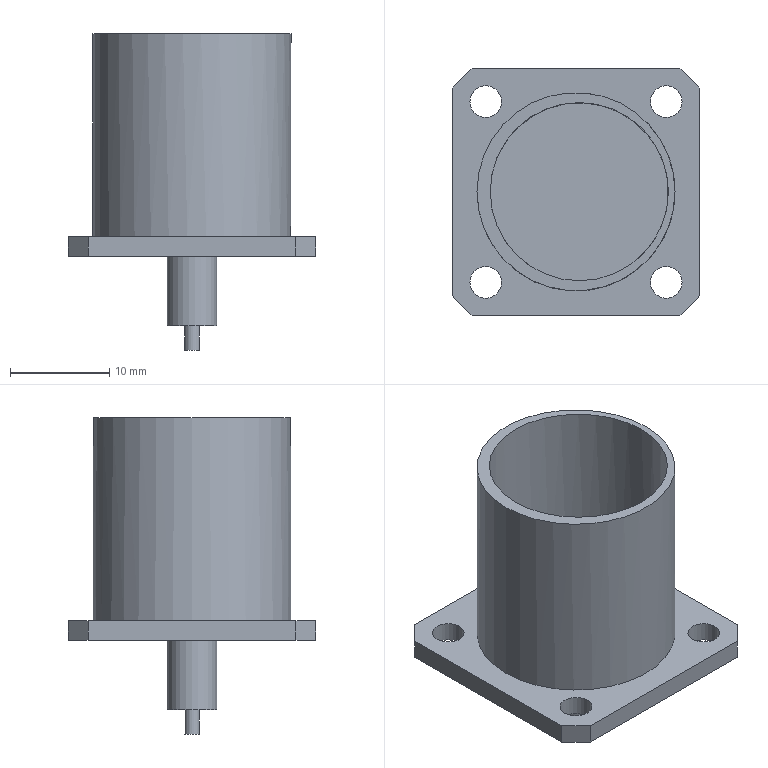Part | STEP file | SOLID | 1 solid | 22 faces | box 25 x 25 x 32 mm | volume 2535 mm3 | plane 14 | cylinder 8 | commonest cylinder face diameters 3.2 x4 1.5 x1 5 x1 18 x1 20 x1